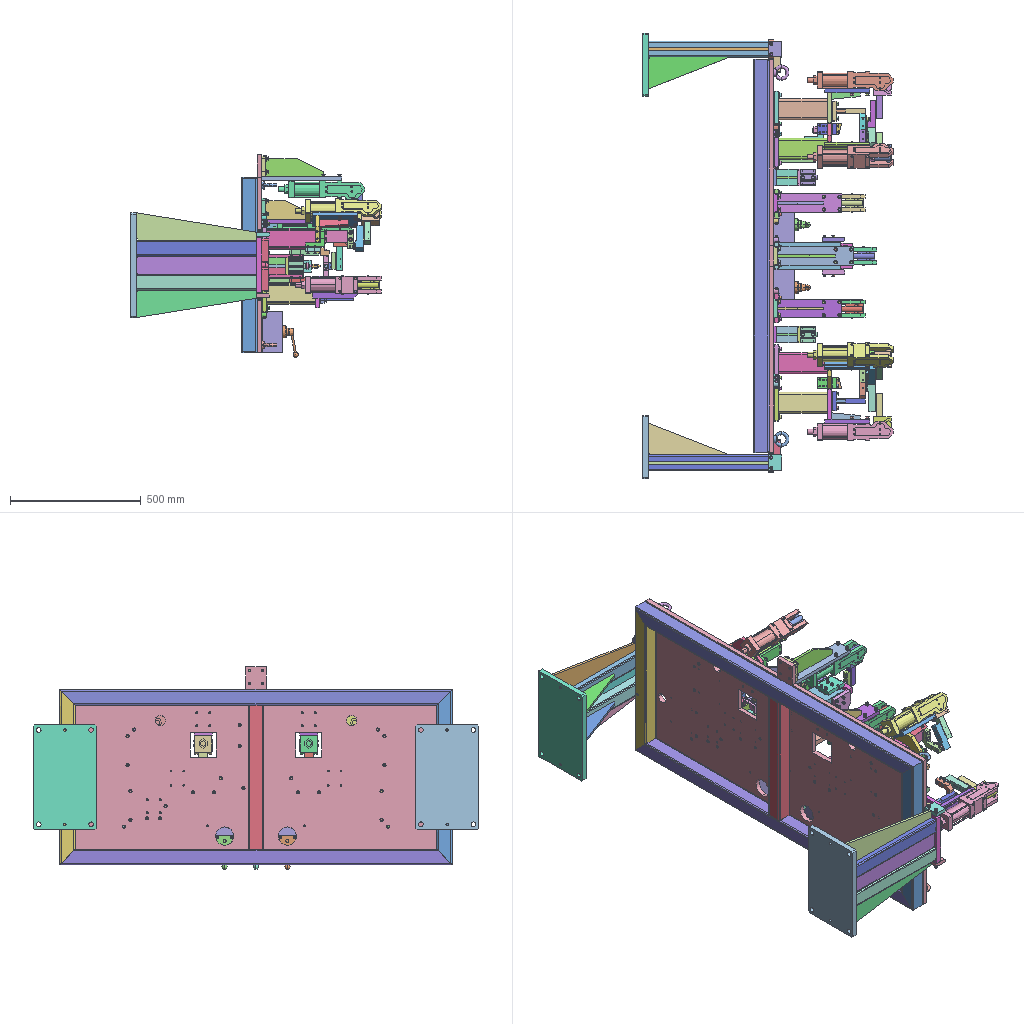Assembly | STEP file | 580 different items | 580 placed | box 956 x 1700 x 774 mm
Parts list (item | name | quantity | parent item | size | volume), first 321 of 580 items:
1 | Positioning_id2322_x_t | x1 | in Positioning_x_t | 31 x 12 x 12 mm | 2751 mm3
2 | Positioning_id2318_x_t | x1 | in Positioning_x_t | 10 x 64 x 70 mm | 43261 mm3
3 | Positioning_id2314_x_t | x1 | in Positioning_x_t | 80 x 6 x 27 mm | 12960 mm3
4 | Positioning_id2310_x_t | x1 | in Positioning_x_t | 10 x 64 x 64 mm | 38415 mm3
5 | Positioning_id2306_x_t | x1 | in Positioning_x_t | 80 x 64 x 10 mm | 51200 mm3
6 | Positioning_id2302_x_t | x1 | in Positioning_x_t | 80 x 6 x 27 mm | 12960 mm3
7 | Positioning_id2298_x_t | x1 | in Positioning_x_t | 68.5 x 64 x 71 mm | 221302 mm3
8 | Positioning_id2294_x_t | x1 | in Positioning_x_t | 80 x 6 x 27 mm | 12960 mm3
9 | Positioning_id2290_x_t | x1 | in Positioning_x_t | 80 x 6 x 27 mm | 12960 mm3
10 | Positioning_id2286_x_t | x1 | in Positioning_x_t | 80 x 64 x 10 mm | 51200 mm3
11 | Positioning_id2282_x_t | x1 | in Positioning_x_t | 10 x 64 x 64 mm | 38415 mm3
12 | Positioning_id2278_x_t | x1 | in Positioning_x_t | 10 x 64 x 70 mm | 43261 mm3
13 | Positioning_id2274_x_t | x1 | in Positioning_x_t | 68.5 x 64 x 71 mm | 221302 mm3
14 | Positioning_id2270_x_t | x1 | in Positioning_x_t | 20 x 77.797 x 69.995 mm | 41126 mm3
15 | Positioning_id2266_x_t | x1 | in Positioning_x_t | 126.002 x 75 x 45 mm | 142700 mm3
16 | Positioning_id2262_x_t | x1 | in Positioning_x_t | 20 x 82.349 x 70.139 mm | 42004 mm3
17 | Positioning_id2258_x_t | x1 | in Positioning_x_t | 126.002 x 75 x 45 mm | 142700 mm3
18 | Positioning_id2254_x_t | x1 | in Positioning_x_t | 20 x 88.297 x 69.995 mm | 43755 mm3
19 | Positioning_id2250_x_t | x1 | in Positioning_x_t | 126.002 x 75 x 45 mm | 142700 mm3
20 | Positioning_id2246_x_t | x1 | in Positioning_x_t | 20 x 82.349 x 70.139 mm | 42004 mm3
21 | Positioning_id2242_x_t | x1 | in Positioning_x_t | 126.002 x 75 x 45 mm | 142700 mm3
22 | Positioning_id2238_x_t | x1 | in Positioning_x_t | 38 x 13 x 13 mm | 2572 mm3
23 | Positioning_id2234_x_t | x1 | in Positioning_x_t | 38 x 13 x 13 mm | 2572 mm3
24 | Positioning_id2230_x_t | x1 | in Positioning_x_t | 38 x 13 x 13 mm | 2572 mm3
25 | Positioning_id2226_x_t | x1 | in Positioning_x_t | 38 x 13 x 13 mm | 2572 mm3
26 | Positioning_id2222_x_t | x1 | in Positioning_x_t | 94.176 x 62 x 127.891 mm | 147960 mm3
27 | Positioning_id2218_x_t | x1 | in Positioning_x_t | 94.176 x 62 x 127.891 mm | 147960 mm3
28 | Positioning_id2214_x_t | x1 | in Positioning_x_t | 80 x 380 x 160 mm | 271642 mm3
29 | Positioning_id2210_x_t | x1 | in Positioning_x_t | 94.176 x 62 x 127.891 mm | 147960 mm3
30 | Positioning_id2206_x_t | x1 | in Positioning_x_t | 40 x 67 x 67 mm | 82781 mm3
31 | Positioning_id2202_x_t | x1 | in Positioning_x_t | 10 x 10 x 31 mm | 1106 mm3
32 | Positioning_id2198_x_t | x1 | in Positioning_x_t | 15 x 15 x 2 mm | 276.46 mm3
33 | Positioning_id2194_x_t | x1 | in Positioning_x_t | 36 x 25 x 15 mm | 6488 mm3
34 | Positioning_id2190_x_t | x1 | in Positioning_x_t | 20 x 20 x 3 mm | 706.858 mm3
35 | Positioning_id2186_x_t | x1 | in Positioning_x_t | 15 x 2 x 15 mm | 276.46 mm3
36 | Positioning_id2182_x_t | x1 | in Positioning_x_t | 20 x 3 x 20 mm | 706.858 mm3
37 | Positioning_id2178_x_t | x1 | in Positioning_x_t | 10 x 31 x 10 mm | 1106 mm3
38 | Positioning_id2174_x_t | x1 | in Positioning_x_t | 36 x 15 x 25 mm | 6488 mm3
39 | Positioning_id2170_x_t | x1 | in Positioning_x_t | 20 x 20 x 3 mm | 706.858 mm3
40 | Positioning_id2166_x_t | x1 | in Positioning_x_t | 10 x 10 x 31 mm | 1106 mm3
41 | Positioning_id2162_x_t | x1 | in Positioning_x_t | 15 x 15 x 2 mm | 276.46 mm3
42 | Positioning_id2158_x_t | x1 | in Positioning_x_t | 36 x 25 x 15 mm | 6488 mm3
43 | Positioning_id2154_x_t | x1 | in Positioning_x_t | 10 x 31 x 10 mm | 1171 mm3
44 | Positioning_id2150_x_t | x1 | in Positioning_x_t | 10 x 31 x 10 mm | 1171 mm3
45 | Positioning_id2146_x_t | x1 | in Positioning_x_t | 50 x 3.35 x 40 mm | 6184 mm3
46 | Positioning_id2142_x_t | x1 | in Positioning_x_t | 85 x 16 x 100 mm | 91411 mm3
47 | Positioning_id2138_x_t | x1 | in Positioning_x_t | 10 x 31 x 10 mm | 1171 mm3
48 | Positioning_id2134_x_t | x1 | in Positioning_x_t | 10 x 31 x 10 mm | 1171 mm3
49 | Positioning_id2130_x_t | x1 | in Positioning_x_t | 175 x 10 x 70 mm | 97500 mm3
50 | Positioning_id2126_x_t | x1 | in Positioning_x_t | 152 x 110 x 86 mm | 594352 mm3
51 | Positioning_id2122_x_t | x1 | in Positioning_x_t | 152 x 110 x 86 mm | 594352 mm3
52 | Positioning_id2118_x_t | x1 | in Positioning_x_t | 15 x 100 x 110 mm | 155502 mm3
53 | Positioning_id2114_x_t | x1 | in Positioning_x_t | 175 x 10 x 70 mm | 97500 mm3
54 | Positioning_id2110_x_t | x1 | in Positioning_x_t | 31 x 17 x 17 mm | 3085 mm3
55 | Positioning_id2106_x_t | x1 | in Positioning_x_t | 31 x 17 x 17 mm | 3085 mm3
56 | Positioning_id2102_x_t | x1 | in Positioning_x_t | 50 x 40 x 3 mm | 5538 mm3
57 | Positioning_id2098_x_t | x1 | in Positioning_x_t | 10 x 10 x 31 mm | 1171 mm3
58 | Positioning_id2094_x_t | x1 | in Positioning_x_t | 10 x 10 x 31 mm | 1171 mm3
59 | Positioning_id2090_x_t | x1 | in Positioning_x_t | 10 x 10 x 31 mm | 1171 mm3
60 | Positioning_id2086_x_t | x1 | in Positioning_x_t | 85 x 66 x 16 mm | 83727 mm3
61 | Positioning_id2082_x_t | x1 | in Positioning_x_t | 10 x 10 x 31 mm | 1171 mm3
62 | Positioning_id2078_x_t | x1 | in Positioning_x_t | 85 x 16 x 100 mm | 91411 mm3
63 | Positioning_id2074_x_t | x1 | in Positioning_x_t | 10 x 31 x 10 mm | 1171 mm3
64 | Positioning_id2070_x_t | x1 | in Positioning_x_t | 50 x 3.35 x 40 mm | 6184 mm3
65 | Positioning_id2066_x_t | x1 | in Positioning_x_t | 236.25 x 100 x 40 mm | 918195 mm3
66 | Positioning_id2062_x_t | x1 | in Positioning_x_t | 10 x 31 x 10 mm | 1171 mm3
67 | Positioning_id2058_x_t | x1 | in Positioning_x_t | 10 x 31 x 10 mm | 1171 mm3
68 | Positioning_id2054_x_t | x1 | in Positioning_x_t | 20 x 3 x 20 mm | 706.858 mm3
69 | Positioning_id2050_x_t | x1 | in Positioning_x_t | 10 x 31 x 10 mm | 1171 mm3
70 | Positioning_id2046_x_t | x1 | in Positioning_x_t | 10 x 31 x 10 mm | 1106 mm3
71 | Positioning_id2042_x_t | x1 | in Positioning_x_t | 43 x 13 x 13 mm | 2687 mm3
72 | Positioning_id2038_x_t | x1 | in Positioning_x_t | 20 x 3 x 20 mm | 706.858 mm3
73 | Positioning_id2034_x_t | x1 | in Positioning_x_t | 3 x 20 x 20 mm | 706.858 mm3
74 | Positioning_id2030_x_t | x1 | in Positioning_x_t | 43 x 13 x 13 mm | 2687 mm3
75 | Positioning_id2026_x_t | x1 | in Positioning_x_t | 36 x 15 x 25 mm | 6488 mm3
76 | Positioning_id2022_x_t | x1 | in Positioning_x_t | 20 x 20 x 3 mm | 706.858 mm3
77 | Positioning_id2018_x_t | x1 | in Positioning_x_t | 43 x 13 x 13 mm | 2687 mm3
78 | Positioning_id2014_x_t | x1 | in Positioning_x_t | 36 x 25 x 15 mm | 6488 mm3
79 | Positioning_id2010_x_t | x1 | in Positioning_x_t | 15 x 15 x 2 mm | 276.46 mm3
80 | Positioning_id2006_x_t | x1 | in Positioning_x_t | 15 x 2 x 15 mm | 276.46 mm3
81 | Positioning_id2002_x_t | x1 | in Positioning_x_t | 43 x 13 x 13 mm | 2687 mm3
82 | Positioning_id1998_x_t | x1 | in Positioning_x_t | 3 x 20 x 20 mm | 706.858 mm3
83 | Positioning_id1994_x_t | x1 | in Positioning_x_t | 10 x 10 x 31 mm | 1106 mm3
84 | Positioning_id1990_x_t | x1 | in Positioning_x_t | 15 x 2 x 15 mm | 276.46 mm3
85 | Positioning_id1986_x_t | x1 | in Positioning_x_t | 3 x 20 x 20 mm | 706.858 mm3
86 | Positioning_id1982_x_t | x1 | in Positioning_x_t | 3 x 86 x 110 mm | 27023 mm3
87 | Positioning_id1978_x_t | x1 | in Positioning_x_t | 10 x 31 x 10 mm | 1106 mm3
88 | Positioning_id1974_x_t | x1 | in Positioning_x_t | 36 x 15 x 25 mm | 6488 mm3
89 | Positioning_id1970_x_t | x1 | in Positioning_x_t | 3 x 20 x 20 mm | 706.858 mm3
90 | Positioning_id1966_x_t | x1 | in Positioning_x_t | 16 x 16 x 36 mm | 4409 mm3
91 | Positioning_id1962_x_t | x1 | in Positioning_x_t | 30 x 20 x 15 mm | 7190 mm3
92 | Positioning_id1958_x_t | x1 | in Positioning_x_t | 15 x 20 x 65 mm | 17144 mm3
93 | Positioning_id1954_x_t | x1 | in Positioning_x_t | 44.8 x 96 x 25 mm | 50269 mm3
94 | Positioning_id1950_x_t | x1 | in Positioning_x_t | 10.1 x 13 x 13 mm | 1181 mm3
95 | Positioning_id1946_x_t | x1 | in Positioning_x_t | 10.1 x 13 x 13 mm | 1181 mm3
96 | Positioning_id1942_x_t | x1 | in Positioning_x_t | 25 x 25 x 90 mm | 49849 mm3
97 | Positioning_id1938_x_t | x1 | in Positioning_x_t | 43 x 13 x 13 mm | 2687 mm3
98 | Positioning_id1934_x_t | x1 | in Positioning_x_t | 43 x 13 x 13 mm | 2687 mm3
99 | Positioning_id1930_x_t | x1 | in Positioning_x_t | 3 x 20 x 20 mm | 706.858 mm3
100 | Positioning_id1926_x_t | x1 | in Positioning_x_t | 15 x 70 x 80 mm | 80048 mm3
101 | Positioning_id1922_x_t | x1 | in Positioning_x_t | 43 x 13 x 13 mm | 2687 mm3
102 | Positioning_id1918_x_t | x1 | in Positioning_x_t | 328 x 72 x 73 mm | 808881 mm3
103 | Positioning_id1914_x_t | x1 | in Positioning_x_t | 6 x 2.5 x 6 mm | 65.686 mm3
104 | Positioning_id1910_x_t | x1 | in Positioning_x_t | 81.5 x 36 x 70 mm | 136244 mm3
105 | Positioning_id1906_x_t | x1 | in Positioning_x_t | 220 x 10 x 70 mm | 129000 mm3
106 | Positioning_id1902_x_t | x1 | in Positioning_x_t | 3 x 20 x 20 mm | 706.858 mm3
107 | Positioning_id1898_x_t | x1 | in Positioning_x_t | 3 x 20 x 20 mm | 706.858 mm3
108 | Positioning_id1894_x_t | x1 | in Positioning_x_t | 3 x 20 x 20 mm | 706.858 mm3
109 | Positioning_id1890_x_t | x1 | in Positioning_x_t | 43 x 13 x 13 mm | 2687 mm3
110 | Positioning_id1886_x_t | x1 | in Positioning_x_t | 13 x 13 x 10.1 mm | 1181 mm3
111 | Positioning_id1882_x_t | x1 | in Positioning_x_t | 13 x 13 x 10.1 mm | 1181 mm3
112 | Positioning_id1878_x_t | x1 | in Positioning_x_t | 305 x 70 x 15 mm | 316433 mm3
113 | Positioning_id1874_x_t | x1 | in Positioning_x_t | 13 x 13 x 10.1 mm | 1181 mm3
114 | Positioning_id1870_x_t | x1 | in Positioning_x_t | 6 x 2.5 x 6 mm | 65.686 mm3
115 | Positioning_id1866_x_t | x1 | in Positioning_x_t | 13 x 13 x 10.1 mm | 1181 mm3
116 | Positioning_id1862_x_t | x1 | in Positioning_x_t | 3 x 20 x 20 mm | 706.858 mm3
117 | Positioning_id1858_x_t | x1 | in Positioning_x_t | 43 x 13 x 13 mm | 2687 mm3
118 | Positioning_id1854_x_t | x1 | in Positioning_x_t | 160 x 70 x 15 mm | 164843 mm3
119 | Positioning_id1850_x_t | x1 | in Positioning_x_t | 43 x 13 x 13 mm | 2687 mm3
120 | Positioning_id1846_x_t | x1 | in Positioning_x_t | 43 x 13 x 13 mm | 2687 mm3
121 | Positioning_id1842_x_t | x1 | in Positioning_x_t | 3 x 20 x 20 mm | 706.858 mm3
122 | Positioning_id1838_x_t | x1 | in Positioning_x_t | 15 x 70 x 80 mm | 79602 mm3
123 | Positioning_id1834_x_t | x1 | in Positioning_x_t | 43 x 13 x 13 mm | 2687 mm3
124 | Positioning_id1830_x_t | x1 | in Positioning_x_t | 70 x 10 x 70 mm | 27875 mm3
125 | Positioning_id1826_x_t | x1 | in Positioning_x_t | 3 x 20 x 20 mm | 706.858 mm3
126 | Positioning_id1822_x_t | x1 | in Positioning_x_t | 3 x 20 x 20 mm | 706.858 mm3
127 | Positioning_id1818_x_t | x1 | in Positioning_x_t | 14.45 x 27.713 x 24 mm | 4910 mm3
128 | Positioning_id1814_x_t | x1 | in Positioning_x_t | 72 x 62 x 45 mm | 93359 mm3
129 | Positioning_id1810_x_t | x1 | in Positioning_x_t | 78 x 25 x 28 mm | 16926 mm3
130 | Positioning_id1806_x_t | x1 | in Positioning_x_t | 110 x 27.049 x 31.474 mm | 33027 mm3
131 | Positioning_id1802_x_t | x1 | in Positioning_x_t | 110 x 25 x 12 mm | 26400 mm3
132 | Positioning_id1798_x_t | x1 | in Positioning_x_t | 110 x 27.049 x 31.474 mm | 33027 mm3
133 | Positioning_id1794_x_t | x1 | in Positioning_x_t | 110 x 25 x 12 mm | 26400 mm3
134 | Positioning_id1790_x_t | x1 | in Positioning_x_t | 31 x 25 x 25 mm | 4491 mm3
135 | Positioning_id1786_x_t | x1 | in Positioning_x_t | 20 x 25 x 25 mm | 3469 mm3
136 | Positioning_id1782_x_t | x1 | in Positioning_x_t | 30.998 x 78.984 x 97.893 mm | 64322 mm3
137 | Positioning_id1778_x_t | x1 | in Positioning_x_t | 10.1 x 13 x 13 mm | 1181 mm3
138 | Positioning_id1774_x_t | x1 | in Positioning_x_t | 3 x 60.629 x 71.68 mm | 3518 mm3
139 | Positioning_id1770_x_t | x1 | in Positioning_x_t | 25 x 72.101 x 88.063 mm | 49849 mm3
140 | Positioning_id1766_x_t | x1 | in Positioning_x_t | 10.1 x 13 x 13 mm | 1181 mm3
141 | Positioning_id1762_x_t | x1 | in Positioning_x_t | 13 x 15.998 x 15.372 mm | 1181 mm3
142 | Positioning_id1758_x_t | x1 | in Positioning_x_t | 13 x 15.998 x 15.372 mm | 1181 mm3
143 | Positioning_id1754_x_t | x1 | in Positioning_x_t | 13 x 15.998 x 15.372 mm | 1181 mm3
144 | Positioning_id1750_x_t | x1 | in Positioning_x_t | 13 x 15.998 x 15.372 mm | 1181 mm3
145 | Positioning_id1746_x_t | x1 | in Positioning_x_t | 328 x 95.116 x 97.081 mm | 808881 mm3
146 | Positioning_id1742_x_t | x1 | in Positioning_x_t | 81.5 x 68.206 x 75.942 mm | 136244 mm3
147 | Positioning_id1738_x_t | x1 | in Positioning_x_t | 171.5 x 65.944 x 52.438 mm | 176258 mm3
148 | Positioning_id1734_x_t | x1 | in Positioning_x_t | 18 x 19.007 x 20.481 mm | 3755 mm3
149 | Positioning_id1730_x_t | x1 | in Positioning_x_t | 6 x 5.097 x 5.956 mm | 61.942 mm3
150 | Positioning_id1726_x_t | x1 | in Positioning_x_t | 6 x 5.097 x 5.956 mm | 61.942 mm3
151 | Positioning_id1722_x_t | x1 | in Positioning_x_t | 6 x 5.489 x 6.349 mm | 65.686 mm3
152 | Positioning_id1718_x_t | x1 | in Positioning_x_t | 6 x 5.489 x 6.349 mm | 65.686 mm3
153 | Positioning_id1714_x_t | x1 | in Positioning_x_t | 15 x 154 x 145 mm | 245583 mm3
154 | Positioning_id1710_x_t | x1 | in Positioning_x_t | 20 x 25 x 25 mm | 3469 mm3
155 | Positioning_id1706_x_t | x1 | in Positioning_x_t | 31 x 25 x 25 mm | 4946 mm3
156 | Positioning_id1702_x_t | x1 | in Positioning_x_t | 30.998 x 111.963 x 25 mm | 61638 mm3
157 | Positioning_id1698_x_t | x1 | in Positioning_x_t | 3 x 70 x 25 mm | 3518 mm3
158 | Positioning_id1694_x_t | x1 | in Positioning_x_t | 328 x 73 x 72 mm | 808881 mm3
159 | Positioning_id1690_x_t | x1 | in Positioning_x_t | 171.5 x 15 x 84 mm | 210585 mm3
160 | Positioning_id1686_x_t | x1 | in Positioning_x_t | 6 x 6 x 2.5 mm | 65.686 mm3
161 | Positioning_id1682_x_t | x1 | in Positioning_x_t | 6 x 6 x 2.5 mm | 61.942 mm3
162 | Positioning_id1678_x_t | x1 | in Positioning_x_t | 6 x 6 x 2.5 mm | 65.686 mm3
163 | Positioning_id1674_x_t | x1 | in Positioning_x_t | 6 x 6 x 2.5 mm | 61.942 mm3
164 | Positioning_id1670_x_t | x1 | in Positioning_x_t | 25 x 90 x 25 mm | 49849 mm3
165 | Positioning_id1666_x_t | x1 | in Positioning_x_t | 13 x 10.1 x 13 mm | 1181 mm3
166 | Positioning_id1662_x_t | x1 | in Positioning_x_t | 13 x 10.1 x 13 mm | 1181 mm3
167 | Positioning_id1658_x_t | x1 | in Positioning_x_t | 13 x 10.1 x 13 mm | 1181 mm3
168 | Positioning_id1654_x_t | x1 | in Positioning_x_t | 13 x 10.1 x 13 mm | 1181 mm3
169 | Positioning_id1650_x_t | x1 | in Positioning_x_t | 81.5 x 70 x 36 mm | 136244 mm3
170 | Positioning_id1646_x_t | x1 | in Positioning_x_t | 38 x 13 x 13 mm | 2572 mm3
171 | Positioning_id1642_x_t | x1 | in Positioning_x_t | 15 x 15 x 2 mm | 276.46 mm3
172 | Positioning_id1638_x_t | x1 | in Positioning_x_t | 3 x 40 x 45 mm | 5400 mm3
173 | Positioning_id1634_x_t | x1 | in Positioning_x_t | 3 x 20 x 20 mm | 706.858 mm3
174 | Positioning_id1630_x_t | x1 | in Positioning_x_t | 3 x 20 x 20 mm | 706.858 mm3
175 | Positioning_id1626_x_t | x1 | in Positioning_x_t | 36 x 15 x 25 mm | 6488 mm3
176 | Positioning_id1622_x_t | x1 | in Positioning_x_t | 10 x 10 x 31 mm | 1106 mm3
177 | Positioning_id1618_x_t | x1 | in Positioning_x_t | 10 x 10 x 31 mm | 1171 mm3
178 | Positioning_id1614_x_t | x1 | in Positioning_x_t | 10.8 x 20.03 x 17.346 mm | 1581 mm3
179 | Positioning_id1610_x_t | x1 | in Positioning_x_t | 12 x 16 x 16 mm | 1877 mm3
180 | Positioning_id1606_x_t | x1 | in Positioning_x_t | 30 x 15 x 25 mm | 9340 mm3
181 | Positioning_id1602_x_t | x1 | in Positioning_x_t | 3 x 20 x 20 mm | 706.858 mm3
182 | Positioning_id1598_x_t | x1 | in Positioning_x_t | 52 x 18.4 x 18.398 mm | 7494 mm3
183 | Positioning_id1594_x_t | x1 | in Positioning_x_t | 36 x 25 x 15 mm | 6488 mm3
184 | Positioning_id1590_x_t | x1 | in Positioning_x_t | 15 x 2 x 15 mm | 276.46 mm3
185 | Positioning_id1586_x_t | x1 | in Positioning_x_t | 3 x 20 x 65 mm | 2438 mm3
186 | Positioning_id1582_x_t | x1 | in Positioning_x_t | 300 x 120 x 10 mm | 189875 mm3
187 | Positioning_id1578_x_t | x1 | in Positioning_x_t | 10 x 31 x 10 mm | 1106 mm3
188 | Positioning_id1574_x_t | x1 | in Positioning_x_t | 20 x 10 x 10 mm | 1571 mm3
189 | Positioning_id1570_x_t | x1 | in Positioning_x_t | 3 x 70 x 25 mm | 3518 mm3
190 | Positioning_id1566_x_t | x1 | in Positioning_x_t | 15 x 140 x 140 mm | 284071 mm3
191 | Positioning_id1562_x_t | x1 | in Positioning_x_t | 3 x 20 x 20 mm | 706.858 mm3
192 | Positioning_id1558_x_t | x1 | in Positioning_x_t | 20 x 3 x 20 mm | 706.858 mm3
193 | Positioning_id1554_x_t | x1 | in Positioning_x_t | 10 x 10 x 31 mm | 1171 mm3
194 | Positioning_id1550_x_t | x1 | in Positioning_x_t | 38 x 13 x 13 mm | 2572 mm3
195 | Positioning_id1546_x_t | x1 | in Positioning_x_t | 3 x 110 x 86 mm | 27023 mm3
196 | Positioning_id1542_x_t | x1 | in Positioning_x_t | 43 x 13 x 13 mm | 2687 mm3
197 | Positioning_id1538_x_t | x1 | in Positioning_x_t | 10 x 31 x 10 mm | 1106 mm3
198 | Positioning_id1534_x_t | x1 | in Positioning_x_t | 36 x 15 x 25 mm | 6488 mm3
199 | Positioning_id1530_x_t | x1 | in Positioning_x_t | 116.841 x 40 x 19.713 mm | 80314 mm3
200 | Positioning_id1526_x_t | x1 | in Positioning_x_t | 43 x 13 x 13 mm | 2687 mm3
201 | Positioning_id1522_x_t | x1 | in Positioning_x_t | 70 x 40 x 67 mm | 66885 mm3
202 | Positioning_id1518_x_t | x1 | in Positioning_x_t | 15 x 164 x 110 mm | 238350 mm3
203 | Positioning_id1514_x_t | x1 | in Positioning_x_t | 3 x 140 x 140 mm | 58800 mm3
204 | Positioning_id1510_x_t | x1 | in Positioning_x_t | 25 x 25 x 90 mm | 49849 mm3
205 | Positioning_id1506_x_t | x1 | in Positioning_x_t | 81.5 x 68.206 x 75.942 mm | 136244 mm3
206 | Positioning_id1502_x_t | x1 | in Positioning_x_t | 3 x 20 x 20 mm | 706.858 mm3
207 | Positioning_id1498_x_t | x1 | in Positioning_x_t | 13 x 13 x 10.1 mm | 1181 mm3
208 | Positioning_id1494_x_t | x1 | in Positioning_x_t | 10.1 x 13 x 13 mm | 1181 mm3
209 | Positioning_id1490_x_t | x1 | in Positioning_x_t | 3 x 20 x 20 mm | 706.858 mm3
210 | Positioning_id1486_x_t | x1 | in Positioning_x_t | 3 x 75 x 50 mm | 11250 mm3
211 | Positioning_id1482_x_t | x1 | in Positioning_x_t | 36 x 15 x 25 mm | 6488 mm3
212 | Positioning_id1478_x_t | x1 | in Positioning_x_t | 20 x 10 x 10 mm | 1571 mm3
213 | Positioning_id1474_x_t | x1 | in Positioning_x_t | 30 x 15 x 25 mm | 9340 mm3
214 | Positioning_id1470_x_t | x1 | in Positioning_x_t | 10 x 10 x 31 mm | 1171 mm3
215 | Positioning_id1466_x_t | x1 | in Positioning_x_t | 6 x 5.489 x 6.349 mm | 65.686 mm3
216 | Positioning_id1462_x_t | x1 | in Positioning_x_t | 3 x 20 x 20 mm | 706.858 mm3
217 | Positioning_id1458_x_t | x1 | in Positioning_x_t | 10 x 10 x 31 mm | 1171 mm3
218 | Positioning_id1454_x_t | x1 | in Positioning_x_t | 10 x 10 x 31 mm | 1171 mm3
219 | Positioning_id1450_x_t | x1 | in Positioning_x_t | 43 x 13 x 13 mm | 2687 mm3
220 | Positioning_id1446_x_t | x1 | in Positioning_x_t | 13 x 13 x 10.1 mm | 1181 mm3
221 | Positioning_id1442_x_t | x1 | in Positioning_x_t | 13 x 10.1 x 13 mm | 1181 mm3
222 | Positioning_id1438_x_t | x1 | in Positioning_x_t | 60 x 60 x 670 mm | 652149 mm3
223 | Positioning_id1434_x_t | x1 | in Positioning_x_t | 31 x 10 x 10 mm | 1171 mm3
224 | Positioning_id1430_x_t | x1 | in Positioning_x_t | 3 x 20 x 20 mm | 706.858 mm3
225 | Positioning_id1426_x_t | x1 | in Positioning_x_t | 10 x 10 x 31 mm | 1171 mm3
226 | Positioning_id1422_x_t | x1 | in Positioning_x_t | 15 x 20 x 65 mm | 17144 mm3
227 | Positioning_id1418_x_t | x1 | in Positioning_x_t | 56.173 x 40 x 15 mm | 30547 mm3
228 | Positioning_id1414_x_t | x1 | in Positioning_x_t | 3 x 20 x 20 mm | 706.858 mm3
229 | Positioning_id1410_x_t | x1 | in Positioning_x_t | 38 x 13 x 13 mm | 2572 mm3
230 | Positioning_id1406_x_t | x1 | in Positioning_x_t | 12 x 16 x 16 mm | 1877 mm3
231 | Positioning_id1402_x_t | x1 | in Positioning_x_t | 15 x 154 x 145 mm | 246102 mm3
232 | Positioning_id1398_x_t | x1 | in Positioning_x_t | 13 x 13 x 10.1 mm | 1181 mm3
233 | Positioning_id1394_x_t | x1 | in Positioning_x_t | 38 x 13 x 13 mm | 2572 mm3
234 | Positioning_id1390_x_t | x1 | in Positioning_x_t | 15 x 2 x 15 mm | 276.46 mm3
235 | Positioning_id1386_x_t | x1 | in Positioning_x_t | 38 x 13 x 13 mm | 2572 mm3
236 | Positioning_id1382_x_t | x1 | in Positioning_x_t | 10 x 31 x 10 mm | 1106 mm3
237 | Positioning_id1378_x_t | x1 | in Positioning_x_t | 56.173 x 40 x 15 mm | 30547 mm3
238 | Positioning_id1374_x_t | x1 | in Positioning_x_t | 3 x 20 x 20 mm | 706.858 mm3
239 | Positioning_id1370_x_t | x1 | in Positioning_x_t | 3 x 20 x 20 mm | 706.858 mm3
240 | Positioning_id1366_x_t | x1 | in Positioning_x_t | 3 x 140 x 140 mm | 58800 mm3
241 | Positioning_id1362_x_t | x1 | in Positioning_x_t | 20 x 25 x 128 mm | 39468 mm3
242 | Positioning_id1358_x_t | x1 | in Positioning_x_t | 10 x 10 x 31 mm | 1171 mm3
243 | Positioning_id1354_x_t | x1 | in Positioning_x_t | 20 x 3 x 20 mm | 706.858 mm3
244 | Positioning_id1350_x_t | x1 | in Positioning_x_t | 43 x 13 x 13 mm | 2687 mm3
245 | Positioning_id1346_x_t | x1 | in Positioning_x_t | 20 x 3 x 20 mm | 706.858 mm3
246 | Positioning_id1342_x_t | x1 | in Positioning_x_t | 15 x 2 x 15 mm | 276.46 mm3
247 | Positioning_id1338_x_t | x1 | in Positioning_x_t | 6 x 2.5 x 6 mm | 65.686 mm3
248 | Positioning_id1334_x_t | x1 | in Positioning_x_t | 60 x 1500 x 60 mm | 1539500 mm3
249 | Positioning_id1330_x_t | x1 | in Positioning_x_t | 50 x 60 x 15 mm | 42341 mm3
250 | Positioning_id1326_x_t | x1 | in Positioning_x_t | 36 x 15 x 25 mm | 6488 mm3
251 | Positioning_id1322_x_t | x1 | in Positioning_x_t | 10.8 x 20.03 x 17.346 mm | 1581 mm3
252 | Positioning_id1318_x_t | x1 | in Positioning_x_t | 6 x 6 x 2.5 mm | 61.942 mm3
253 | Positioning_id1314_x_t | x1 | in Positioning_x_t | 10 x 10 x 31 mm | 1106 mm3
254 | Positioning_id1310_x_t | x1 | in Positioning_x_t | 38 x 13 x 13 mm | 2572 mm3
255 | Positioning_id1306_x_t | x1 | in Positioning_x_t | 6 x 5.097 x 5.956 mm | 61.942 mm3
256 | Positioning_id1302_x_t | x1 | in Positioning_x_t | 10 x 10 x 31 mm | 1171 mm3
257 | Positioning_id1298_x_t | x1 | in Positioning_x_t | 13 x 13 x 10.1 mm | 1181 mm3
258 | Positioning_id1294_x_t | x1 | in Positioning_x_t | 43 x 13 x 13 mm | 2687 mm3
259 | Positioning_id1290_x_t | x1 | in Positioning_x_t | 30.998 x 106.963 x 25 mm | 67424 mm3
260 | Positioning_id1286_x_t | x1 | in Positioning_x_t | 13 x 13 x 10.1 mm | 1181 mm3
261 | Positioning_id1282_x_t | x1 | in Positioning_x_t | 3 x 20 x 20 mm | 706.858 mm3
262 | Positioning_id1278_x_t | x1 | in Positioning_x_t | 38 x 13 x 13 mm | 2572 mm3
263 | Positioning_id1274_x_t | x1 | in Positioning_x_t | 10.1 x 13 x 13 mm | 1181 mm3
264 | Positioning_id1270_x_t | x1 | in Positioning_x_t | 38 x 13 x 13 mm | 2572 mm3
265 | Positioning_id1266_x_t | x1 | in Positioning_x_t | 43 x 13 x 13 mm | 2687 mm3
266 | Positioning_id1262_x_t | x1 | in Positioning_x_t | 43 x 13 x 13 mm | 2687 mm3
267 | Positioning_id1258_x_t | x1 | in Positioning_x_t | 328 x 72 x 73 mm | 808881 mm3
268 | Positioning_id1254_x_t | x1 | in Positioning_x_t | 45 x 40 x 3 mm | 5400 mm3
269 | Positioning_id1250_x_t | x1 | in Positioning_x_t | 20 x 20 x 3 mm | 706.858 mm3
270 | Positioning_id1246_x_t | x1 | in Positioning_x_t | 43 x 13 x 13 mm | 2687 mm3
271 | Positioning_id1242_x_t | x1 | in Positioning_x_t | 20 x 25 x 128 mm | 39468 mm3
272 | Positioning_id1238_x_t | x1 | in Positioning_x_t | 50 x 60 x 15 mm | 42341 mm3
273 | Positioning_id1234_x_t | x1 | in Positioning_x_t | 43 x 13 x 13 mm | 2687 mm3
274 | Positioning_id1230_x_t | x1 | in Positioning_x_t | 36 x 25 x 15 mm | 6488 mm3
275 | Positioning_id1226_x_t | x1 | in Positioning_x_t | 10 x 31 x 10 mm | 1106 mm3
276 | Positioning_id1222_x_t | x1 | in Positioning_x_t | 15 x 2 x 15 mm | 276.46 mm3
277 | Positioning_id1218_x_t | x1 | in Positioning_x_t | 20 x 20 x 3 mm | 706.858 mm3
278 | Positioning_id1214_x_t | x1 | in Positioning_x_t | 13 x 15.998 x 15.372 mm | 1181 mm3
279 | Positioning_id1210_x_t | x1 | in Positioning_x_t | 15 x 75 x 65 mm | 68460 mm3
280 | Positioning_id1206_x_t | x1 | in Positioning_x_t | 16 x 5 x 16 mm | 1005 mm3
281 | Positioning_id1202_x_t | x1 | in Positioning_x_t | 43 x 13 x 13 mm | 2687 mm3
282 | Positioning_id1198_x_t | x1 | in Positioning_x_t | 50 x 40 x 3 mm | 5538 mm3
283 | Positioning_id1194_x_t | x1 | in Positioning_x_t | 36 x 25 x 15 mm | 6488 mm3
284 | Positioning_id1190_x_t | x1 | in Positioning_x_t | 20 x 3 x 20 mm | 706.858 mm3
285 | Positioning_id1186_x_t | x1 | in Positioning_x_t | 43 x 13 x 13 mm | 2687 mm3
286 | Positioning_id1182_x_t | x1 | in Positioning_x_t | 300 x 120 x 10 mm | 189875 mm3
287 | Positioning_id1178_x_t | x1 | in Positioning_x_t | 43 x 13 x 13 mm | 2687 mm3
288 | Positioning_id1174_x_t | x1 | in Positioning_x_t | 43 x 13 x 13 mm | 2687 mm3
289 | Positioning_id1170_x_t | x1 | in Positioning_x_t | 10.1 x 13 x 13 mm | 1181 mm3
290 | Positioning_id1166_x_t | x1 | in Positioning_x_t | 20 x 20 x 3 mm | 706.858 mm3
291 | Positioning_id1162_x_t | x1 | in Positioning_x_t | 10.1 x 13 x 13 mm | 1181 mm3
292 | Positioning_id1158_x_t | x1 | in Positioning_x_t | 43 x 13 x 13 mm | 2687 mm3
293 | Positioning_id1154_x_t | x1 | in Positioning_x_t | 20 x 3 x 20 mm | 706.858 mm3
294 | Positioning_id1150_x_t | x1 | in Positioning_x_t | 31 x 10 x 10 mm | 1171 mm3
295 | Positioning_id1146_x_t | x1 | in Positioning_x_t | 20 x 20 x 3 mm | 706.858 mm3
296 | Positioning_id1142_x_t | x1 | in Positioning_x_t | 3 x 20 x 20 mm | 706.858 mm3
297 | Positioning_id1138_x_t | x1 | in Positioning_x_t | 31 x 10 x 10 mm | 1171 mm3
298 | Positioning_id1134_x_t | x1 | in Positioning_x_t | 20 x 25 x 25 mm | 3469 mm3
299 | Positioning_id1130_x_t | x1 | in Positioning_x_t | 328 x 95.116 x 97.081 mm | 808881 mm3
300 | Positioning_id1126_x_t | x1 | in Positioning_x_t | 13 x 13 x 10.1 mm | 1181 mm3
301 | Positioning_id1122_x_t | x1 | in Positioning_x_t | 10 x 10 x 31 mm | 1171 mm3
302 | Positioning_id1118_x_t | x1 | in Positioning_x_t | 52 x 18.4 x 18.398 mm | 7494 mm3
303 | Positioning_id1114_x_t | x1 | in Positioning_x_t | 36 x 25 x 15 mm | 6488 mm3
304 | Positioning_id1110_x_t | x1 | in Positioning_x_t | 3 x 140 x 140 mm | 58800 mm3
305 | Positioning_id1106_x_t | x1 | in Positioning_x_t | 13 x 10.1 x 13 mm | 1181 mm3
306 | Positioning_id1102_x_t | x1 | in Positioning_x_t | 460 x 10 x 70 mm | 321000 mm3
307 | Positioning_id1098_x_t | x1 | in Positioning_x_t | 25 x 100 x 200 mm | 444348 mm3
308 | Positioning_id1094_x_t | x1 | in Positioning_x_t | 36 x 25 x 15 mm | 6488 mm3
309 | Positioning_id1090_x_t | x1 | in Positioning_x_t | 3 x 20 x 20 mm | 706.858 mm3
310 | Positioning_id1086_x_t | x1 | in Positioning_x_t | 80 x 58 x 29.1 mm | 23470 mm3
311 | Positioning_id1082_x_t | x1 | in Positioning_x_t | 80 x 58 x 29.1 mm | 23470 mm3
312 | Positioning_id1078_x_t | x1 | in Positioning_x_t | 15 x 140 x 140 mm | 284071 mm3
313 | Positioning_id1074_x_t | x1 | in Positioning_x_t | 43 x 13 x 13 mm | 2687 mm3
314 | Positioning_id1070_x_t | x1 | in Positioning_x_t | 52 x 18.4 x 18.398 mm | 7494 mm3
315 | Positioning_id1066_x_t | x1 | in Positioning_x_t | 38 x 13 x 13 mm | 2572 mm3
316 | Positioning_id1062_x_t | x1 | in Positioning_x_t | 50 x 60 x 15 mm | 42341 mm3
317 | Positioning_id1058_x_t | x1 | in Positioning_x_t | 31 x 10 x 10 mm | 1171 mm3
318 | Positioning_id1054_x_t | x1 | in Positioning_x_t | 52 x 18.4 x 18.398 mm | 7494 mm3
319 | Positioning_id1050_x_t | x1 | in Positioning_x_t | 36 x 25 x 15 mm | 6488 mm3
320 | Positioning_id1046_x_t | x1 | in Positioning_x_t | 6 x 2.5 x 6 mm | 65.686 mm3
321 | Positioning_id1042_x_t | x1 | in Positioning_x_t | 20 x 3 x 20 mm | 706.858 mm3
Placements (level | parent | child | x y z in mm | rotation matrix by rows), first 222 of 580 lines:
1 | Positioning_x_t | Positioning_id2322_x_t | 0.0 0.0 0.0 | 1 0 0 0 1 0 0 0 1
1 | Positioning_x_t | Positioning_id2318_x_t | 0.0 0.0 0.0 | 1 0 0 0 1 0 0 0 1
1 | Positioning_x_t | Positioning_id2314_x_t | 0.0 0.0 0.0 | 1 0 0 0 1 0 0 0 1
1 | Positioning_x_t | Positioning_id2310_x_t | 0.0 0.0 0.0 | 1 0 0 0 1 0 0 0 1
1 | Positioning_x_t | Positioning_id2306_x_t | 0.0 0.0 0.0 | 1 0 0 0 1 0 0 0 1
1 | Positioning_x_t | Positioning_id2302_x_t | 0.0 0.0 0.0 | 1 0 0 0 1 0 0 0 1
1 | Positioning_x_t | Positioning_id2298_x_t | 0.0 0.0 0.0 | 1 0 0 0 1 0 0 0 1
1 | Positioning_x_t | Positioning_id2294_x_t | 0.0 0.0 0.0 | 1 0 0 0 1 0 0 0 1
1 | Positioning_x_t | Positioning_id2290_x_t | 0.0 0.0 0.0 | 1 0 0 0 1 0 0 0 1
1 | Positioning_x_t | Positioning_id2286_x_t | 0.0 0.0 0.0 | 1 0 0 0 1 0 0 0 1
1 | Positioning_x_t | Positioning_id2282_x_t | 0.0 0.0 0.0 | 1 0 0 0 1 0 0 0 1
1 | Positioning_x_t | Positioning_id2278_x_t | 0.0 0.0 0.0 | 1 0 0 0 1 0 0 0 1
1 | Positioning_x_t | Positioning_id2274_x_t | 0.0 0.0 0.0 | 1 0 0 0 1 0 0 0 1
1 | Positioning_x_t | Positioning_id2270_x_t | 0.0 0.0 0.0 | 1 0 0 0 1 0 0 0 1
1 | Positioning_x_t | Positioning_id2266_x_t | 0.0 0.0 0.0 | 1 0 0 0 1 0 0 0 1
1 | Positioning_x_t | Positioning_id2262_x_t | 0.0 0.0 0.0 | 1 0 0 0 1 0 0 0 1
1 | Positioning_x_t | Positioning_id2258_x_t | 0.0 0.0 0.0 | 1 0 0 0 1 0 0 0 1
1 | Positioning_x_t | Positioning_id2254_x_t | 0.0 0.0 0.0 | 1 0 0 0 1 0 0 0 1
1 | Positioning_x_t | Positioning_id2250_x_t | 0.0 0.0 0.0 | 1 0 0 0 1 0 0 0 1
1 | Positioning_x_t | Positioning_id2246_x_t | 0.0 0.0 0.0 | 1 0 0 0 1 0 0 0 1
1 | Positioning_x_t | Positioning_id2242_x_t | 0.0 0.0 0.0 | 1 0 0 0 1 0 0 0 1
1 | Positioning_x_t | Positioning_id2238_x_t | 0.0 0.0 0.0 | 1 0 0 0 1 0 0 0 1
1 | Positioning_x_t | Positioning_id2234_x_t | 0.0 0.0 0.0 | 1 0 0 0 1 0 0 0 1
1 | Positioning_x_t | Positioning_id2230_x_t | 0.0 0.0 0.0 | 1 0 0 0 1 0 0 0 1
1 | Positioning_x_t | Positioning_id2226_x_t | 0.0 0.0 0.0 | 1 0 0 0 1 0 0 0 1
1 | Positioning_x_t | Positioning_id2222_x_t | 0.0 0.0 0.0 | 1 0 0 0 1 0 0 0 1
1 | Positioning_x_t | Positioning_id2218_x_t | 0.0 0.0 0.0 | 1 0 0 0 1 0 0 0 1
1 | Positioning_x_t | Positioning_id2214_x_t | 0.0 0.0 0.0 | 1 0 0 0 1 0 0 0 1
1 | Positioning_x_t | Positioning_id2210_x_t | 0.0 0.0 0.0 | 1 0 0 0 1 0 0 0 1
1 | Positioning_x_t | Positioning_id2206_x_t | 0.0 0.0 0.0 | 1 0 0 0 1 0 0 0 1
1 | Positioning_x_t | Positioning_id2202_x_t | 0.0 0.0 0.0 | 1 0 0 0 1 0 0 0 1
1 | Positioning_x_t | Positioning_id2198_x_t | 0.0 0.0 0.0 | 1 0 0 0 1 0 0 0 1
1 | Positioning_x_t | Positioning_id2194_x_t | 0.0 0.0 0.0 | 1 0 0 0 1 0 0 0 1
1 | Positioning_x_t | Positioning_id2190_x_t | 0.0 0.0 0.0 | 1 0 0 0 1 0 0 0 1
1 | Positioning_x_t | Positioning_id2186_x_t | 0.0 0.0 0.0 | 1 0 0 0 1 0 0 0 1
1 | Positioning_x_t | Positioning_id2182_x_t | 0.0 0.0 0.0 | 1 0 0 0 1 0 0 0 1
1 | Positioning_x_t | Positioning_id2178_x_t | 0.0 0.0 0.0 | 1 0 0 0 1 0 0 0 1
1 | Positioning_x_t | Positioning_id2174_x_t | 0.0 0.0 0.0 | 1 0 0 0 1 0 0 0 1
1 | Positioning_x_t | Positioning_id2170_x_t | 0.0 0.0 0.0 | 1 0 0 0 1 0 0 0 1
1 | Positioning_x_t | Positioning_id2166_x_t | 0.0 0.0 0.0 | 1 0 0 0 1 0 0 0 1
1 | Positioning_x_t | Positioning_id2162_x_t | 0.0 0.0 0.0 | 1 0 0 0 1 0 0 0 1
1 | Positioning_x_t | Positioning_id2158_x_t | 0.0 0.0 0.0 | 1 0 0 0 1 0 0 0 1
1 | Positioning_x_t | Positioning_id2154_x_t | 0.0 0.0 0.0 | 1 0 0 0 1 0 0 0 1
1 | Positioning_x_t | Positioning_id2150_x_t | 0.0 0.0 0.0 | 1 0 0 0 1 0 0 0 1
1 | Positioning_x_t | Positioning_id2146_x_t | 0.0 0.0 0.0 | 1 0 0 0 1 0 0 0 1
1 | Positioning_x_t | Positioning_id2142_x_t | 0.0 0.0 0.0 | 1 0 0 0 1 0 0 0 1
1 | Positioning_x_t | Positioning_id2138_x_t | 0.0 0.0 0.0 | 1 0 0 0 1 0 0 0 1
1 | Positioning_x_t | Positioning_id2134_x_t | 0.0 0.0 0.0 | 1 0 0 0 1 0 0 0 1
1 | Positioning_x_t | Positioning_id2130_x_t | 0.0 0.0 0.0 | 1 0 0 0 1 0 0 0 1
1 | Positioning_x_t | Positioning_id2126_x_t | 0.0 0.0 0.0 | 1 0 0 0 1 0 0 0 1
1 | Positioning_x_t | Positioning_id2122_x_t | 0.0 0.0 0.0 | 1 0 0 0 1 0 0 0 1
1 | Positioning_x_t | Positioning_id2118_x_t | 0.0 0.0 0.0 | 1 0 0 0 1 0 0 0 1
1 | Positioning_x_t | Positioning_id2114_x_t | 0.0 0.0 0.0 | 1 0 0 0 1 0 0 0 1
1 | Positioning_x_t | Positioning_id2110_x_t | 0.0 0.0 0.0 | 1 0 0 0 1 0 0 0 1
1 | Positioning_x_t | Positioning_id2106_x_t | 0.0 0.0 0.0 | 1 0 0 0 1 0 0 0 1
1 | Positioning_x_t | Positioning_id2102_x_t | 0.0 0.0 0.0 | 1 0 0 0 1 0 0 0 1
1 | Positioning_x_t | Positioning_id2098_x_t | 0.0 0.0 0.0 | 1 0 0 0 1 0 0 0 1
1 | Positioning_x_t | Positioning_id2094_x_t | 0.0 0.0 0.0 | 1 0 0 0 1 0 0 0 1
1 | Positioning_x_t | Positioning_id2090_x_t | 0.0 0.0 0.0 | 1 0 0 0 1 0 0 0 1
1 | Positioning_x_t | Positioning_id2086_x_t | 0.0 0.0 0.0 | 1 0 0 0 1 0 0 0 1
1 | Positioning_x_t | Positioning_id2082_x_t | 0.0 0.0 0.0 | 1 0 0 0 1 0 0 0 1
1 | Positioning_x_t | Positioning_id2078_x_t | 0.0 0.0 0.0 | 1 0 0 0 1 0 0 0 1
1 | Positioning_x_t | Positioning_id2074_x_t | 0.0 0.0 0.0 | 1 0 0 0 1 0 0 0 1
1 | Positioning_x_t | Positioning_id2070_x_t | 0.0 0.0 0.0 | 1 0 0 0 1 0 0 0 1
1 | Positioning_x_t | Positioning_id2066_x_t | 0.0 0.0 0.0 | 1 0 0 0 1 0 0 0 1
1 | Positioning_x_t | Positioning_id2062_x_t | 0.0 0.0 0.0 | 1 0 0 0 1 0 0 0 1
1 | Positioning_x_t | Positioning_id2058_x_t | 0.0 0.0 0.0 | 1 0 0 0 1 0 0 0 1
1 | Positioning_x_t | Positioning_id2054_x_t | 0.0 0.0 0.0 | 1 0 0 0 1 0 0 0 1
1 | Positioning_x_t | Positioning_id2050_x_t | 0.0 0.0 0.0 | 1 0 0 0 1 0 0 0 1
1 | Positioning_x_t | Positioning_id2046_x_t | 0.0 0.0 0.0 | 1 0 0 0 1 0 0 0 1
1 | Positioning_x_t | Positioning_id2042_x_t | 0.0 0.0 0.0 | 1 0 0 0 1 0 0 0 1
1 | Positioning_x_t | Positioning_id2038_x_t | 0.0 0.0 0.0 | 1 0 0 0 1 0 0 0 1
1 | Positioning_x_t | Positioning_id2034_x_t | 0.0 0.0 0.0 | 1 0 0 0 1 0 0 0 1
1 | Positioning_x_t | Positioning_id2030_x_t | 0.0 0.0 0.0 | 1 0 0 0 1 0 0 0 1
1 | Positioning_x_t | Positioning_id2026_x_t | 0.0 0.0 0.0 | 1 0 0 0 1 0 0 0 1
1 | Positioning_x_t | Positioning_id2022_x_t | 0.0 0.0 0.0 | 1 0 0 0 1 0 0 0 1
1 | Positioning_x_t | Positioning_id2018_x_t | 0.0 0.0 0.0 | 1 0 0 0 1 0 0 0 1
1 | Positioning_x_t | Positioning_id2014_x_t | 0.0 0.0 0.0 | 1 0 0 0 1 0 0 0 1
1 | Positioning_x_t | Positioning_id2010_x_t | 0.0 0.0 0.0 | 1 0 0 0 1 0 0 0 1
1 | Positioning_x_t | Positioning_id2006_x_t | 0.0 0.0 0.0 | 1 0 0 0 1 0 0 0 1
1 | Positioning_x_t | Positioning_id2002_x_t | 0.0 0.0 0.0 | 1 0 0 0 1 0 0 0 1
1 | Positioning_x_t | Positioning_id1998_x_t | 0.0 0.0 0.0 | 1 0 0 0 1 0 0 0 1
1 | Positioning_x_t | Positioning_id1994_x_t | 0.0 0.0 0.0 | 1 0 0 0 1 0 0 0 1
1 | Positioning_x_t | Positioning_id1990_x_t | 0.0 0.0 0.0 | 1 0 0 0 1 0 0 0 1
1 | Positioning_x_t | Positioning_id1986_x_t | 0.0 0.0 0.0 | 1 0 0 0 1 0 0 0 1
1 | Positioning_x_t | Positioning_id1982_x_t | 0.0 0.0 0.0 | 1 0 0 0 1 0 0 0 1
1 | Positioning_x_t | Positioning_id1978_x_t | 0.0 0.0 0.0 | 1 0 0 0 1 0 0 0 1
1 | Positioning_x_t | Positioning_id1974_x_t | 0.0 0.0 0.0 | 1 0 0 0 1 0 0 0 1
1 | Positioning_x_t | Positioning_id1970_x_t | 0.0 0.0 0.0 | 1 0 0 0 1 0 0 0 1
1 | Positioning_x_t | Positioning_id1966_x_t | 0.0 0.0 0.0 | 1 0 0 0 1 0 0 0 1
1 | Positioning_x_t | Positioning_id1962_x_t | 0.0 0.0 0.0 | 1 0 0 0 1 0 0 0 1
1 | Positioning_x_t | Positioning_id1958_x_t | 0.0 0.0 0.0 | 1 0 0 0 1 0 0 0 1
1 | Positioning_x_t | Positioning_id1954_x_t | 0.0 0.0 0.0 | 1 0 0 0 1 0 0 0 1
1 | Positioning_x_t | Positioning_id1950_x_t | 0.0 0.0 0.0 | 1 0 0 0 1 0 0 0 1
1 | Positioning_x_t | Positioning_id1946_x_t | 0.0 0.0 0.0 | 1 0 0 0 1 0 0 0 1
1 | Positioning_x_t | Positioning_id1942_x_t | 0.0 0.0 0.0 | 1 0 0 0 1 0 0 0 1
1 | Positioning_x_t | Positioning_id1938_x_t | 0.0 0.0 0.0 | 1 0 0 0 1 0 0 0 1
1 | Positioning_x_t | Positioning_id1934_x_t | 0.0 0.0 0.0 | 1 0 0 0 1 0 0 0 1
1 | Positioning_x_t | Positioning_id1930_x_t | 0.0 0.0 0.0 | 1 0 0 0 1 0 0 0 1
1 | Positioning_x_t | Positioning_id1926_x_t | 0.0 0.0 0.0 | 1 0 0 0 1 0 0 0 1
1 | Positioning_x_t | Positioning_id1922_x_t | 0.0 0.0 0.0 | 1 0 0 0 1 0 0 0 1
1 | Positioning_x_t | Positioning_id1918_x_t | 0.0 0.0 0.0 | 1 0 0 0 1 0 0 0 1
1 | Positioning_x_t | Positioning_id1914_x_t | 0.0 0.0 0.0 | 1 0 0 0 1 0 0 0 1
1 | Positioning_x_t | Positioning_id1910_x_t | 0.0 0.0 0.0 | 1 0 0 0 1 0 0 0 1
1 | Positioning_x_t | Positioning_id1906_x_t | 0.0 0.0 0.0 | 1 0 0 0 1 0 0 0 1
1 | Positioning_x_t | Positioning_id1902_x_t | 0.0 0.0 0.0 | 1 0 0 0 1 0 0 0 1
1 | Positioning_x_t | Positioning_id1898_x_t | 0.0 0.0 0.0 | 1 0 0 0 1 0 0 0 1
1 | Positioning_x_t | Positioning_id1894_x_t | 0.0 0.0 0.0 | 1 0 0 0 1 0 0 0 1
1 | Positioning_x_t | Positioning_id1890_x_t | 0.0 0.0 0.0 | 1 0 0 0 1 0 0 0 1
1 | Positioning_x_t | Positioning_id1886_x_t | 0.0 0.0 0.0 | 1 0 0 0 1 0 0 0 1
1 | Positioning_x_t | Positioning_id1882_x_t | 0.0 0.0 0.0 | 1 0 0 0 1 0 0 0 1
1 | Positioning_x_t | Positioning_id1878_x_t | 0.0 0.0 0.0 | 1 0 0 0 1 0 0 0 1
1 | Positioning_x_t | Positioning_id1874_x_t | 0.0 0.0 0.0 | 1 0 0 0 1 0 0 0 1
1 | Positioning_x_t | Positioning_id1870_x_t | 0.0 0.0 0.0 | 1 0 0 0 1 0 0 0 1
1 | Positioning_x_t | Positioning_id1866_x_t | 0.0 0.0 0.0 | 1 0 0 0 1 0 0 0 1
1 | Positioning_x_t | Positioning_id1862_x_t | 0.0 0.0 0.0 | 1 0 0 0 1 0 0 0 1
1 | Positioning_x_t | Positioning_id1858_x_t | 0.0 0.0 0.0 | 1 0 0 0 1 0 0 0 1
1 | Positioning_x_t | Positioning_id1854_x_t | 0.0 0.0 0.0 | 1 0 0 0 1 0 0 0 1
1 | Positioning_x_t | Positioning_id1850_x_t | 0.0 0.0 0.0 | 1 0 0 0 1 0 0 0 1
1 | Positioning_x_t | Positioning_id1846_x_t | 0.0 0.0 0.0 | 1 0 0 0 1 0 0 0 1
1 | Positioning_x_t | Positioning_id1842_x_t | 0.0 0.0 0.0 | 1 0 0 0 1 0 0 0 1
1 | Positioning_x_t | Positioning_id1838_x_t | 0.0 0.0 0.0 | 1 0 0 0 1 0 0 0 1
1 | Positioning_x_t | Positioning_id1834_x_t | 0.0 0.0 0.0 | 1 0 0 0 1 0 0 0 1
1 | Positioning_x_t | Positioning_id1830_x_t | 0.0 0.0 0.0 | 1 0 0 0 1 0 0 0 1
1 | Positioning_x_t | Positioning_id1826_x_t | 0.0 0.0 0.0 | 1 0 0 0 1 0 0 0 1
1 | Positioning_x_t | Positioning_id1822_x_t | 0.0 0.0 0.0 | 1 0 0 0 1 0 0 0 1
1 | Positioning_x_t | Positioning_id1818_x_t | 0.0 0.0 0.0 | 1 0 0 0 1 0 0 0 1
1 | Positioning_x_t | Positioning_id1814_x_t | 0.0 0.0 0.0 | 1 0 0 0 1 0 0 0 1
1 | Positioning_x_t | Positioning_id1810_x_t | 0.0 0.0 0.0 | 1 0 0 0 1 0 0 0 1
1 | Positioning_x_t | Positioning_id1806_x_t | 0.0 0.0 0.0 | 1 0 0 0 1 0 0 0 1
1 | Positioning_x_t | Positioning_id1802_x_t | 0.0 0.0 0.0 | 1 0 0 0 1 0 0 0 1
1 | Positioning_x_t | Positioning_id1798_x_t | 0.0 0.0 0.0 | 1 0 0 0 1 0 0 0 1
1 | Positioning_x_t | Positioning_id1794_x_t | 0.0 0.0 0.0 | 1 0 0 0 1 0 0 0 1
1 | Positioning_x_t | Positioning_id1790_x_t | 0.0 0.0 0.0 | 1 0 0 0 1 0 0 0 1
1 | Positioning_x_t | Positioning_id1786_x_t | 0.0 0.0 0.0 | 1 0 0 0 1 0 0 0 1
1 | Positioning_x_t | Positioning_id1782_x_t | 0.0 0.0 0.0 | 1 0 0 0 1 0 0 0 1
1 | Positioning_x_t | Positioning_id1778_x_t | 0.0 0.0 0.0 | 1 0 0 0 1 0 0 0 1
1 | Positioning_x_t | Positioning_id1774_x_t | 0.0 0.0 0.0 | 1 0 0 0 1 0 0 0 1
1 | Positioning_x_t | Positioning_id1770_x_t | 0.0 0.0 0.0 | 1 0 0 0 1 0 0 0 1
1 | Positioning_x_t | Positioning_id1766_x_t | 0.0 0.0 0.0 | 1 0 0 0 1 0 0 0 1
1 | Positioning_x_t | Positioning_id1762_x_t | 0.0 0.0 0.0 | 1 0 0 0 1 0 0 0 1
1 | Positioning_x_t | Positioning_id1758_x_t | 0.0 0.0 0.0 | 1 0 0 0 1 0 0 0 1
1 | Positioning_x_t | Positioning_id1754_x_t | 0.0 0.0 0.0 | 1 0 0 0 1 0 0 0 1
1 | Positioning_x_t | Positioning_id1750_x_t | 0.0 0.0 0.0 | 1 0 0 0 1 0 0 0 1
1 | Positioning_x_t | Positioning_id1746_x_t | 0.0 0.0 0.0 | 1 0 0 0 1 0 0 0 1
1 | Positioning_x_t | Positioning_id1742_x_t | 0.0 0.0 0.0 | 1 0 0 0 1 0 0 0 1
1 | Positioning_x_t | Positioning_id1738_x_t | 0.0 0.0 0.0 | 1 0 0 0 1 0 0 0 1
1 | Positioning_x_t | Positioning_id1734_x_t | 0.0 0.0 0.0 | 1 0 0 0 1 0 0 0 1
1 | Positioning_x_t | Positioning_id1730_x_t | 0.0 0.0 0.0 | 1 0 0 0 1 0 0 0 1
1 | Positioning_x_t | Positioning_id1726_x_t | 0.0 0.0 0.0 | 1 0 0 0 1 0 0 0 1
1 | Positioning_x_t | Positioning_id1722_x_t | 0.0 0.0 0.0 | 1 0 0 0 1 0 0 0 1
1 | Positioning_x_t | Positioning_id1718_x_t | 0.0 0.0 0.0 | 1 0 0 0 1 0 0 0 1
1 | Positioning_x_t | Positioning_id1714_x_t | 0.0 0.0 0.0 | 1 0 0 0 1 0 0 0 1
1 | Positioning_x_t | Positioning_id1710_x_t | 0.0 0.0 0.0 | 1 0 0 0 1 0 0 0 1
1 | Positioning_x_t | Positioning_id1706_x_t | 0.0 0.0 0.0 | 1 0 0 0 1 0 0 0 1
1 | Positioning_x_t | Positioning_id1702_x_t | 0.0 0.0 0.0 | 1 0 0 0 1 0 0 0 1
1 | Positioning_x_t | Positioning_id1698_x_t | 0.0 0.0 0.0 | 1 0 0 0 1 0 0 0 1
1 | Positioning_x_t | Positioning_id1694_x_t | 0.0 0.0 0.0 | 1 0 0 0 1 0 0 0 1
1 | Positioning_x_t | Positioning_id1690_x_t | 0.0 0.0 0.0 | 1 0 0 0 1 0 0 0 1
1 | Positioning_x_t | Positioning_id1686_x_t | 0.0 0.0 0.0 | 1 0 0 0 1 0 0 0 1
1 | Positioning_x_t | Positioning_id1682_x_t | 0.0 0.0 0.0 | 1 0 0 0 1 0 0 0 1
1 | Positioning_x_t | Positioning_id1678_x_t | 0.0 0.0 0.0 | 1 0 0 0 1 0 0 0 1
1 | Positioning_x_t | Positioning_id1674_x_t | 0.0 0.0 0.0 | 1 0 0 0 1 0 0 0 1
1 | Positioning_x_t | Positioning_id1670_x_t | 0.0 0.0 0.0 | 1 0 0 0 1 0 0 0 1
1 | Positioning_x_t | Positioning_id1666_x_t | 0.0 0.0 0.0 | 1 0 0 0 1 0 0 0 1
1 | Positioning_x_t | Positioning_id1662_x_t | 0.0 0.0 0.0 | 1 0 0 0 1 0 0 0 1
1 | Positioning_x_t | Positioning_id1658_x_t | 0.0 0.0 0.0 | 1 0 0 0 1 0 0 0 1
1 | Positioning_x_t | Positioning_id1654_x_t | 0.0 0.0 0.0 | 1 0 0 0 1 0 0 0 1
1 | Positioning_x_t | Positioning_id1650_x_t | 0.0 0.0 0.0 | 1 0 0 0 1 0 0 0 1
1 | Positioning_x_t | Positioning_id1646_x_t | 0.0 0.0 0.0 | 1 0 0 0 1 0 0 0 1
1 | Positioning_x_t | Positioning_id1642_x_t | 0.0 0.0 0.0 | 1 0 0 0 1 0 0 0 1
1 | Positioning_x_t | Positioning_id1638_x_t | 0.0 0.0 0.0 | 1 0 0 0 1 0 0 0 1
1 | Positioning_x_t | Positioning_id1634_x_t | 0.0 0.0 0.0 | 1 0 0 0 1 0 0 0 1
1 | Positioning_x_t | Positioning_id1630_x_t | 0.0 0.0 0.0 | 1 0 0 0 1 0 0 0 1
1 | Positioning_x_t | Positioning_id1626_x_t | 0.0 0.0 0.0 | 1 0 0 0 1 0 0 0 1
1 | Positioning_x_t | Positioning_id1622_x_t | 0.0 0.0 0.0 | 1 0 0 0 1 0 0 0 1
1 | Positioning_x_t | Positioning_id1618_x_t | 0.0 0.0 0.0 | 1 0 0 0 1 0 0 0 1
1 | Positioning_x_t | Positioning_id1614_x_t | 0.0 0.0 0.0 | 1 0 0 0 1 0 0 0 1
1 | Positioning_x_t | Positioning_id1610_x_t | 0.0 0.0 0.0 | 1 0 0 0 1 0 0 0 1
1 | Positioning_x_t | Positioning_id1606_x_t | 0.0 0.0 0.0 | 1 0 0 0 1 0 0 0 1
1 | Positioning_x_t | Positioning_id1602_x_t | 0.0 0.0 0.0 | 1 0 0 0 1 0 0 0 1
1 | Positioning_x_t | Positioning_id1598_x_t | 0.0 0.0 0.0 | 1 0 0 0 1 0 0 0 1
1 | Positioning_x_t | Positioning_id1594_x_t | 0.0 0.0 0.0 | 1 0 0 0 1 0 0 0 1
1 | Positioning_x_t | Positioning_id1590_x_t | 0.0 0.0 0.0 | 1 0 0 0 1 0 0 0 1
1 | Positioning_x_t | Positioning_id1586_x_t | 0.0 0.0 0.0 | 1 0 0 0 1 0 0 0 1
1 | Positioning_x_t | Positioning_id1582_x_t | 0.0 0.0 0.0 | 1 0 0 0 1 0 0 0 1
1 | Positioning_x_t | Positioning_id1578_x_t | 0.0 0.0 0.0 | 1 0 0 0 1 0 0 0 1
1 | Positioning_x_t | Positioning_id1574_x_t | 0.0 0.0 0.0 | 1 0 0 0 1 0 0 0 1
1 | Positioning_x_t | Positioning_id1570_x_t | 0.0 0.0 0.0 | 1 0 0 0 1 0 0 0 1
1 | Positioning_x_t | Positioning_id1566_x_t | 0.0 0.0 0.0 | 1 0 0 0 1 0 0 0 1
1 | Positioning_x_t | Positioning_id1562_x_t | 0.0 0.0 0.0 | 1 0 0 0 1 0 0 0 1
1 | Positioning_x_t | Positioning_id1558_x_t | 0.0 0.0 0.0 | 1 0 0 0 1 0 0 0 1
1 | Positioning_x_t | Positioning_id1554_x_t | 0.0 0.0 0.0 | 1 0 0 0 1 0 0 0 1
1 | Positioning_x_t | Positioning_id1550_x_t | 0.0 0.0 0.0 | 1 0 0 0 1 0 0 0 1
1 | Positioning_x_t | Positioning_id1546_x_t | 0.0 0.0 0.0 | 1 0 0 0 1 0 0 0 1
1 | Positioning_x_t | Positioning_id1542_x_t | 0.0 0.0 0.0 | 1 0 0 0 1 0 0 0 1
1 | Positioning_x_t | Positioning_id1538_x_t | 0.0 0.0 0.0 | 1 0 0 0 1 0 0 0 1
1 | Positioning_x_t | Positioning_id1534_x_t | 0.0 0.0 0.0 | 1 0 0 0 1 0 0 0 1
1 | Positioning_x_t | Positioning_id1530_x_t | 0.0 0.0 0.0 | 1 0 0 0 1 0 0 0 1
1 | Positioning_x_t | Positioning_id1526_x_t | 0.0 0.0 0.0 | 1 0 0 0 1 0 0 0 1
1 | Positioning_x_t | Positioning_id1522_x_t | 0.0 0.0 0.0 | 1 0 0 0 1 0 0 0 1
1 | Positioning_x_t | Positioning_id1518_x_t | 0.0 0.0 0.0 | 1 0 0 0 1 0 0 0 1
1 | Positioning_x_t | Positioning_id1514_x_t | 0.0 0.0 0.0 | 1 0 0 0 1 0 0 0 1
1 | Positioning_x_t | Positioning_id1510_x_t | 0.0 0.0 0.0 | 1 0 0 0 1 0 0 0 1
1 | Positioning_x_t | Positioning_id1506_x_t | 0.0 0.0 0.0 | 1 0 0 0 1 0 0 0 1
1 | Positioning_x_t | Positioning_id1502_x_t | 0.0 0.0 0.0 | 1 0 0 0 1 0 0 0 1
1 | Positioning_x_t | Positioning_id1498_x_t | 0.0 0.0 0.0 | 1 0 0 0 1 0 0 0 1
1 | Positioning_x_t | Positioning_id1494_x_t | 0.0 0.0 0.0 | 1 0 0 0 1 0 0 0 1
1 | Positioning_x_t | Positioning_id1490_x_t | 0.0 0.0 0.0 | 1 0 0 0 1 0 0 0 1
1 | Positioning_x_t | Positioning_id1486_x_t | 0.0 0.0 0.0 | 1 0 0 0 1 0 0 0 1
1 | Positioning_x_t | Positioning_id1482_x_t | 0.0 0.0 0.0 | 1 0 0 0 1 0 0 0 1
1 | Positioning_x_t | Positioning_id1478_x_t | 0.0 0.0 0.0 | 1 0 0 0 1 0 0 0 1
1 | Positioning_x_t | Positioning_id1474_x_t | 0.0 0.0 0.0 | 1 0 0 0 1 0 0 0 1
1 | Positioning_x_t | Positioning_id1470_x_t | 0.0 0.0 0.0 | 1 0 0 0 1 0 0 0 1
1 | Positioning_x_t | Positioning_id1466_x_t | 0.0 0.0 0.0 | 1 0 0 0 1 0 0 0 1
1 | Positioning_x_t | Positioning_id1462_x_t | 0.0 0.0 0.0 | 1 0 0 0 1 0 0 0 1
1 | Positioning_x_t | Positioning_id1458_x_t | 0.0 0.0 0.0 | 1 0 0 0 1 0 0 0 1
1 | Positioning_x_t | Positioning_id1454_x_t | 0.0 0.0 0.0 | 1 0 0 0 1 0 0 0 1
1 | Positioning_x_t | Positioning_id1450_x_t | 0.0 0.0 0.0 | 1 0 0 0 1 0 0 0 1
1 | Positioning_x_t | Positioning_id1446_x_t | 0.0 0.0 0.0 | 1 0 0 0 1 0 0 0 1
1 | Positioning_x_t | Positioning_id1442_x_t | 0.0 0.0 0.0 | 1 0 0 0 1 0 0 0 1
1 | Positioning_x_t | Positioning_id1438_x_t | 0.0 0.0 0.0 | 1 0 0 0 1 0 0 0 1